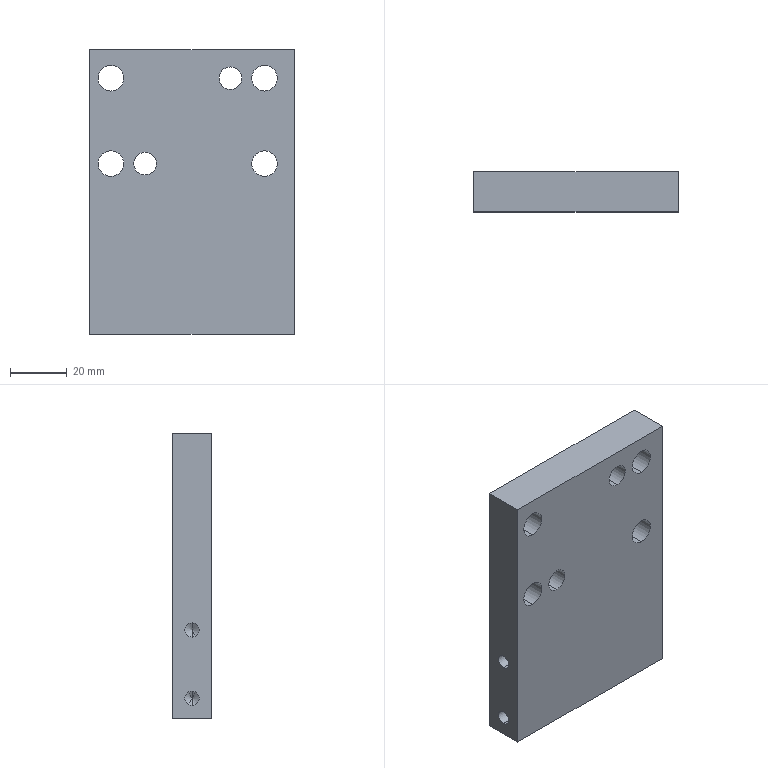Part | STEP file | OP10-139_base plate (F)-R | 1 solid | 34 faces | box 72 x 14 x 100 mm | volume 94613 mm3 | cylinder 20 | cone 8 | plane 6 | commonest cylinder face diameters 5 x8 9 x8 8 x4